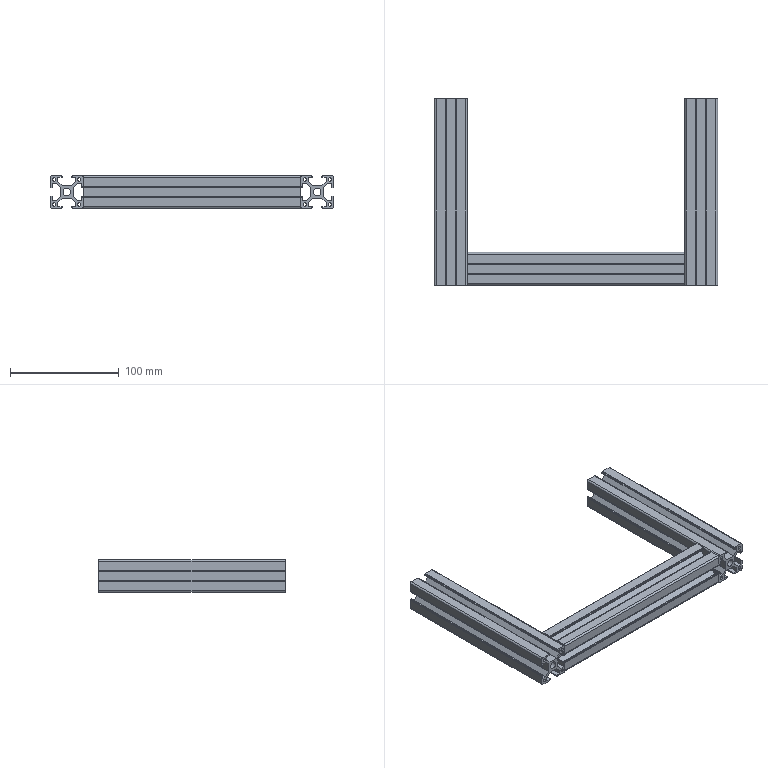Part | SolidWorks | features WeldMemberFeat 1, WeldmentFeature 1 | 3 solids | 228 faces | box 260 x 171 x 30 mm | volume 182154 mm3 | plane 186 | cylinder 42 | commonest cylinder face diameters 3 x36 6.8 x6